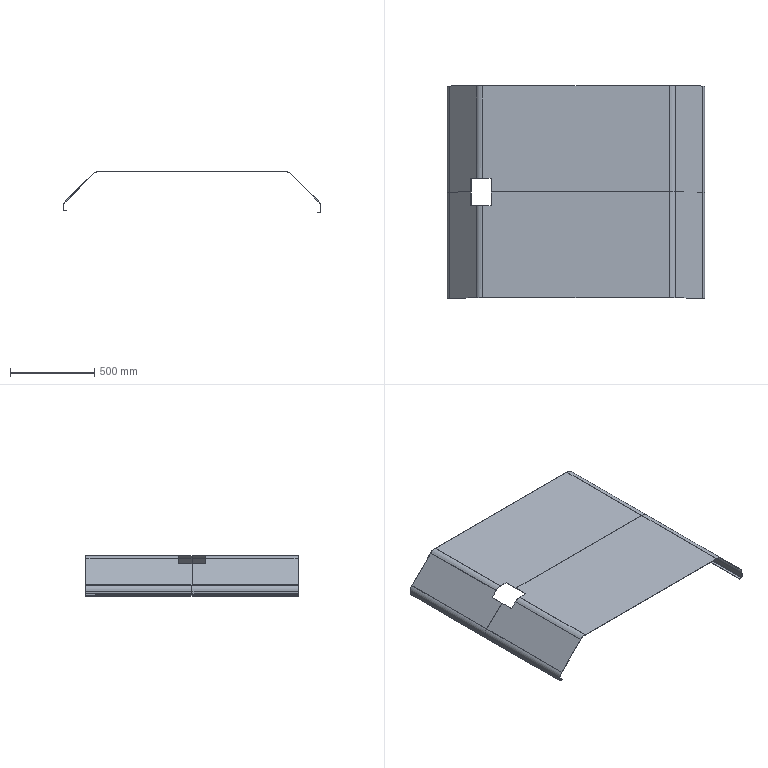Part | NX | features BREP 1 | 1 solid | 87 faces | box 1528 x 1258 x 243.035 mm | volume 4478605 mm3 | plane 61 | spline 17 | cylinder 9 | commonest cylinder face diameters 6 x4 4 x2 10 x2 8 x1